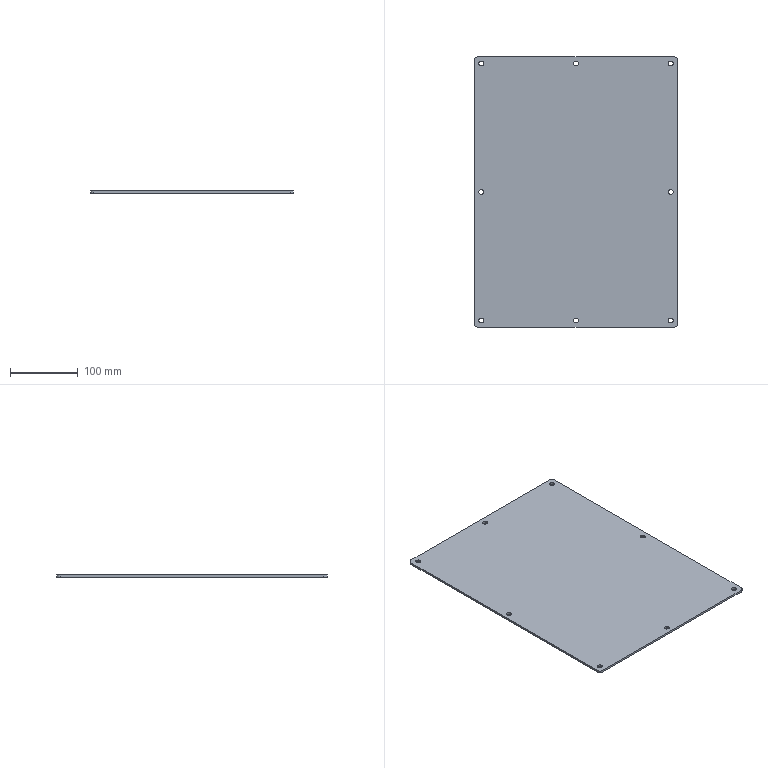Part | SolidWorks | features BaseBody 1 | 1 solid | 26 faces | box 300 x 400 x 3 mm | volume 359012 mm3 | cylinder 20 | plane 6 | commonest cylinder face diameters 7 x16 10 x4
STEP:
#1=CARTESIAN_POINT('',(136.5,-190.,0.));
#2=VERTEX_POINT('',#1);
#3=CARTESIAN_POINT('',(143.5,-190.,0.));
#4=VERTEX_POINT('',#3);
#5=CARTESIAN_POINT('',(140.,-190.,0.));
#6=DIRECTION('',(0.,0.,1.));
#7=DIRECTION('',(1.,0.,0.));
#8=AXIS2_PLACEMENT_3D('',#5,#6,#7);
#9=CIRCLE('',#8,3.5);
#10=EDGE_CURVE('',#2,#4,#9,.T.);
#11=ORIENTED_EDGE('',*,*,#10,.F.);
#12=CARTESIAN_POINT('',(136.5,-190.,3.));
#13=VERTEX_POINT('',#12);
#14=CARTESIAN_POINT('',(136.5,-190.,3.));
#15=DIRECTION('',(0.,0.,1.));
#16=VECTOR('',#15,1000.);
#17=LINE('',#14,#16);
#18=EDGE_CURVE('',#2,#13,#17,.T.);
#19=ORIENTED_EDGE('',*,*,#18,.T.);
#20=CARTESIAN_POINT('',(143.5,-190.,3.));
#21=VERTEX_POINT('',#20);
#22=CARTESIAN_POINT('',(140.,-190.,3.));
#23=DIRECTION('',(0.,0.,1.));
#24=DIRECTION('',(1.,0.,0.));
#25=AXIS2_PLACEMENT_3D('',#22,#23,#24);
#26=CIRCLE('',#25,3.5);
#27=EDGE_CURVE('',#13,#21,#26,.T.);
#28=ORIENTED_EDGE('',*,*,#27,.T.);
#29=CARTESIAN_POINT('',(143.5,-190.,3.));
#30=DIRECTION('',(0.,0.,1.));
#31=VECTOR('',#30,1000.);
#32=LINE('',#29,#31);
#33=EDGE_CURVE('',#4,#21,#32,.T.);
#34=ORIENTED_EDGE('',*,*,#33,.F.);
#35=EDGE_LOOP('',(#11,#19,#28,#34));
#36=FACE_OUTER_BOUND('',#35,.T.);
#37=CARTESIAN_POINT('',(140.,-190.,3.));
#38=DIRECTION('',(0.,0.,1.));
#39=DIRECTION('',(1.,0.,0.));
#40=AXIS2_PLACEMENT_3D('',#37,#38,#39);
#41=CYLINDRICAL_SURFACE('',#40,3.5);
#42=ADVANCED_FACE('',(#36),#41,.F.);
#43=CARTESIAN_POINT('',(-143.5,190.,0.));
#44=VERTEX_POINT('',#43);
#45=CARTESIAN_POINT('',(-136.5,190.,0.));
#46=VERTEX_POINT('',#45);
#47=CARTESIAN_POINT('',(-140.,190.,0.));
#48=DIRECTION('',(0.,0.,1.));
#49=DIRECTION('',(1.,0.,0.));
#50=AXIS2_PLACEMENT_3D('',#47,#48,#49);
#51=CIRCLE('',#50,3.5);
#52=EDGE_CURVE('',#44,#46,#51,.T.);
#53=ORIENTED_EDGE('',*,*,#52,.F.);
#54=CARTESIAN_POINT('',(-143.5,190.,3.));
#55=VERTEX_POINT('',#54);
#56=CARTESIAN_POINT('',(-143.5,190.,3.));
#57=DIRECTION('',(0.,0.,1.));
#58=VECTOR('',#57,1000.);
#59=LINE('',#56,#58);
#60=EDGE_CURVE('',#44,#55,#59,.T.);
#61=ORIENTED_EDGE('',*,*,#60,.T.);
#62=CARTESIAN_POINT('',(-136.5,190.,3.));
#63=VERTEX_POINT('',#62);
#64=CARTESIAN_POINT('',(-140.,190.,3.));
#65=DIRECTION('',(0.,0.,1.));
#66=DIRECTION('',(1.,0.,0.));
#67=AXIS2_PLACEMENT_3D('',#64,#65,#66);
#68=CIRCLE('',#67,3.5);
#69=EDGE_CURVE('',#55,#63,#68,.T.);
#70=ORIENTED_EDGE('',*,*,#69,.T.);
#71=CARTESIAN_POINT('',(-136.5,190.,3.));
#72=DIRECTION('',(0.,0.,1.));
#73=VECTOR('',#72,1000.);
#74=LINE('',#71,#73);
#75=EDGE_CURVE('',#46,#63,#74,.T.);
#76=ORIENTED_EDGE('',*,*,#75,.F.);
#77=EDGE_LOOP('',(#53,#61,#70,#76));
#78=FACE_OUTER_BOUND('',#77,.T.);
#79=CARTESIAN_POINT('',(-140.,190.,3.));
#80=DIRECTION('',(0.,0.,1.));
#81=DIRECTION('',(1.,0.,0.));
#82=AXIS2_PLACEMENT_3D('',#79,#80,#81);
#83=CYLINDRICAL_SURFACE('',#82,3.5);
#84=ADVANCED_FACE('',(#78),#83,.F.);
#85=CARTESIAN_POINT('',(-143.5,-190.,0.));
#86=VERTEX_POINT('',#85);
#87=CARTESIAN_POINT('',(-136.5,-190.,0.));
#88=VERTEX_POINT('',#87);
#89=CARTESIAN_POINT('',(-140.,-190.,0.));
#90=DIRECTION('',(0.,0.,1.));
#91=DIRECTION('',(1.,0.,0.));
#92=AXIS2_PLACEMENT_3D('',#89,#90,#91);
#93=CIRCLE('',#92,3.5);
#94=EDGE_CURVE('',#86,#88,#93,.T.);
#95=ORIENTED_EDGE('',*,*,#94,.F.);
#96=CARTESIAN_POINT('',(-143.5,-190.,3.));
#97=VERTEX_POINT('',#96);
#98=CARTESIAN_POINT('',(-143.5,-190.,3.));
#99=DIRECTION('',(0.,0.,1.));
#100=VECTOR('',#99,1000.);
#101=LINE('',#98,#100);
#102=EDGE_CURVE('',#86,#97,#101,.T.);
#103=ORIENTED_EDGE('',*,*,#102,.T.);
#104=CARTESIAN_POINT('',(-136.5,-190.,3.));
#105=VERTEX_POINT('',#104);
#106=CARTESIAN_POINT('',(-140.,-190.,3.));
#107=DIRECTION('',(0.,0.,1.));
#108=DIRECTION('',(1.,0.,0.));
#109=AXIS2_PLACEMENT_3D('',#106,#107,#108);
#110=CIRCLE('',#109,3.5);
#111=EDGE_CURVE('',#97,#105,#110,.T.);
#112=ORIENTED_EDGE('',*,*,#111,.T.);
#113=CARTESIAN_POINT('',(-136.5,-190.,3.));
#114=DIRECTION('',(0.,0.,1.));
#115=VECTOR('',#114,1000.);
#116=LINE('',#113,#115);
#117=EDGE_CURVE('',#88,#105,#116,.T.);
#118=ORIENTED_EDGE('',*,*,#117,.F.);
#119=EDGE_LOOP('',(#95,#103,#112,#118));
#120=FACE_OUTER_BOUND('',#119,.T.);
#121=CARTESIAN_POINT('',(-140.,-190.,3.));
#122=DIRECTION('',(0.,0.,1.));
#123=DIRECTION('',(1.,0.,0.));
#124=AXIS2_PLACEMENT_3D('',#121,#122,#123);
#125=CYLINDRICAL_SURFACE('',#124,3.5);
#126=ADVANCED_FACE('',(#120),#125,.F.);
#127=CARTESIAN_POINT('',(136.5,190.,0.));
#128=VERTEX_POINT('',#127);
#129=CARTESIAN_POINT('',(143.5,190.,0.));
#130=VERTEX_POINT('',#129);
#131=CARTESIAN_POINT('',(140.,190.,0.));
#132=DIRECTION('',(0.,0.,1.));
#133=DIRECTION('',(1.,0.,0.));
#134=AXIS2_PLACEMENT_3D('',#131,#132,#133);
#135=CIRCLE('',#134,3.5);
#136=EDGE_CURVE('',#128,#130,#135,.T.);
#137=ORIENTED_EDGE('',*,*,#136,.F.);
#138=CARTESIAN_POINT('',(136.5,190.,3.));
#139=VERTEX_POINT('',#138);
#140=CARTESIAN_POINT('',(136.5,190.,3.));
#141=DIRECTION('',(0.,0.,1.));
#142=VECTOR('',#141,1000.);
#143=LINE('',#140,#142);
#144=EDGE_CURVE('',#128,#139,#143,.T.);
#145=ORIENTED_EDGE('',*,*,#144,.T.);
#146=CARTESIAN_POINT('',(143.5,190.,3.));
#147=VERTEX_POINT('',#146);
#148=CARTESIAN_POINT('',(140.,190.,3.));
#149=DIRECTION('',(0.,0.,1.));
#150=DIRECTION('',(1.,0.,0.));
#151=AXIS2_PLACEMENT_3D('',#148,#149,#150);
#152=CIRCLE('',#151,3.5);
#153=EDGE_CURVE('',#139,#147,#152,.T.);
#154=ORIENTED_EDGE('',*,*,#153,.T.);
#155=CARTESIAN_POINT('',(143.5,190.,3.));
#156=DIRECTION('',(0.,0.,1.));
#157=VECTOR('',#156,1000.);
#158=LINE('',#155,#157);
#159=EDGE_CURVE('',#130,#147,#158,.T.);
#160=ORIENTED_EDGE('',*,*,#159,.F.);
#161=EDGE_LOOP('',(#137,#145,#154,#160));
#162=FACE_OUTER_BOUND('',#161,.T.);
#163=CARTESIAN_POINT('',(140.,190.,3.));
#164=DIRECTION('',(0.,0.,1.));
#165=DIRECTION('',(1.,0.,0.));
#166=AXIS2_PLACEMENT_3D('',#163,#164,#165);
#167=CYLINDRICAL_SURFACE('',#166,3.5);
#168=ADVANCED_FACE('',(#162),#167,.F.);
#169=CARTESIAN_POINT('',(-3.5,190.,0.));
#170=VERTEX_POINT('',#169);
#171=CARTESIAN_POINT('',(3.5,190.,0.));
#172=VERTEX_POINT('',#171);
#173=CARTESIAN_POINT('',(0.,190.,0.));
#174=DIRECTION('',(0.,0.,1.));
#175=DIRECTION('',(1.,0.,0.));
#176=AXIS2_PLACEMENT_3D('',#173,#174,#175);
#177=CIRCLE('',#176,3.5);
#178=EDGE_CURVE('',#170,#172,#177,.T.);
#179=ORIENTED_EDGE('',*,*,#178,.F.);
#180=CARTESIAN_POINT('',(-3.5,190.,3.));
#181=VERTEX_POINT('',#180);
#182=CARTESIAN_POINT('',(-3.5,190.,3.));
#183=DIRECTION('',(0.,0.,1.));
#184=VECTOR('',#183,1000.);
#185=LINE('',#182,#184);
#186=EDGE_CURVE('',#170,#181,#185,.T.);
#187=ORIENTED_EDGE('',*,*,#186,.T.);
#188=CARTESIAN_POINT('',(3.5,190.,3.));
#189=VERTEX_POINT('',#188);
#190=CARTESIAN_POINT('',(0.,190.,3.));
#191=DIRECTION('',(0.,0.,1.));
#192=DIRECTION('',(1.,0.,0.));
#193=AXIS2_PLACEMENT_3D('',#190,#191,#192);
#194=CIRCLE('',#193,3.5);
#195=EDGE_CURVE('',#181,#189,#194,.T.);
#196=ORIENTED_EDGE('',*,*,#195,.T.);
#197=CARTESIAN_POINT('',(3.5,190.,3.));
#198=DIRECTION('',(0.,0.,1.));
#199=VECTOR('',#198,1000.);
#200=LINE('',#197,#199);
#201=EDGE_CURVE('',#172,#189,#200,.T.);
#202=ORIENTED_EDGE('',*,*,#201,.F.);
#203=EDGE_LOOP('',(#179,#187,#196,#202));
#204=FACE_OUTER_BOUND('',#203,.T.);
#205=CARTESIAN_POINT('',(0.,190.,3.));
#206=DIRECTION('',(0.,0.,1.));
#207=DIRECTION('',(1.,0.,0.));
#208=AXIS2_PLACEMENT_3D('',#205,#206,#207);
#209=CYLINDRICAL_SURFACE('',#208,3.5);
#210=ADVANCED_FACE('',(#204),#209,.F.);
#211=CARTESIAN_POINT('',(-3.5,-190.,0.));
#212=VERTEX_POINT('',#211);
#213=CARTESIAN_POINT('',(3.5,-190.,0.));
#214=VERTEX_POINT('',#213);
#215=CARTESIAN_POINT('',(0.,-190.,0.));
#216=DIRECTION('',(0.,0.,1.));
#217=DIRECTION('',(1.,0.,0.));
#218=AXIS2_PLACEMENT_3D('',#215,#216,#217);
#219=CIRCLE('',#218,3.5);
#220=EDGE_CURVE('',#212,#214,#219,.T.);
#221=ORIENTED_EDGE('',*,*,#220,.F.);
#222=CARTESIAN_POINT('',(-3.5,-190.,3.));
#223=VERTEX_POINT('',#222);
#224=CARTESIAN_POINT('',(-3.5,-190.,3.));
#225=DIRECTION('',(0.,0.,1.));
#226=VECTOR('',#225,1000.);
#227=LINE('',#224,#226);
#228=EDGE_CURVE('',#212,#223,#227,.T.);
#229=ORIENTED_EDGE('',*,*,#228,.T.);
#230=CARTESIAN_POINT('',(3.5,-190.,3.));
#231=VERTEX_POINT('',#230);
#232=CARTESIAN_POINT('',(0.,-190.,3.));
#233=DIRECTION('',(0.,0.,1.));
#234=DIRECTION('',(1.,0.,0.));
#235=AXIS2_PLACEMENT_3D('',#232,#233,#234);
#236=CIRCLE('',#235,3.5);
#237=EDGE_CURVE('',#223,#231,#236,.T.);
#238=ORIENTED_EDGE('',*,*,#237,.T.);
#239=CARTESIAN_POINT('',(3.5,-190.,3.));
#240=DIRECTION('',(0.,0.,1.));
#241=VECTOR('',#240,1000.);
#242=LINE('',#239,#241);
#243=EDGE_CURVE('',#214,#231,#242,.T.);
#244=ORIENTED_EDGE('',*,*,#243,.F.);
#245=EDGE_LOOP('',(#221,#229,#238,#244));
#246=FACE_OUTER_BOUND('',#245,.T.);
#247=CARTESIAN_POINT('',(0.,-190.,3.));
#248=DIRECTION('',(0.,0.,1.));
#249=DIRECTION('',(1.,0.,0.));
#250=AXIS2_PLACEMENT_3D('',#247,#248,#249);
#251=CYLINDRICAL_SURFACE('',#250,3.5);
#252=ADVANCED_FACE('',(#246),#251,.F.);
#253=CARTESIAN_POINT('',(-143.5,0.,0.));
#254=VERTEX_POINT('',#253);
#255=CARTESIAN_POINT('',(-136.5,0.,0.));
#256=VERTEX_POINT('',#255);
#257=CARTESIAN_POINT('',(-140.,0.,0.));
#258=DIRECTION('',(0.,0.,1.));
#259=DIRECTION('',(1.,0.,0.));
#260=AXIS2_PLACEMENT_3D('',#257,#258,#259);
#261=CIRCLE('',#260,3.5);
#262=EDGE_CURVE('',#254,#256,#261,.T.);
#263=ORIENTED_EDGE('',*,*,#262,.F.);
#264=CARTESIAN_POINT('',(-143.5,0.,3.));
#265=VERTEX_POINT('',#264);
#266=CARTESIAN_POINT('',(-143.5,0.,3.));
#267=DIRECTION('',(0.,0.,1.));
#268=VECTOR('',#267,1000.);
#269=LINE('',#266,#268);
#270=EDGE_CURVE('',#254,#265,#269,.T.);
#271=ORIENTED_EDGE('',*,*,#270,.T.);
#272=CARTESIAN_POINT('',(-136.5,0.,3.));
#273=VERTEX_POINT('',#272);
#274=CARTESIAN_POINT('',(-140.,0.,3.));
#275=DIRECTION('',(0.,0.,1.));
#276=DIRECTION('',(1.,0.,0.));
#277=AXIS2_PLACEMENT_3D('',#274,#275,#276);
#278=CIRCLE('',#277,3.5);
#279=EDGE_CURVE('',#265,#273,#278,.T.);
#280=ORIENTED_EDGE('',*,*,#279,.T.);
#281=CARTESIAN_POINT('',(-136.5,0.,3.));
#282=DIRECTION('',(0.,0.,1.));
#283=VECTOR('',#282,1000.);
#284=LINE('',#281,#283);
#285=EDGE_CURVE('',#256,#273,#284,.T.);
#286=ORIENTED_EDGE('',*,*,#285,.F.);
#287=EDGE_LOOP('',(#263,#271,#280,#286));
#288=FACE_OUTER_BOUND('',#287,.T.);
#289=CARTESIAN_POINT('',(-140.,0.,3.));
#290=DIRECTION('',(0.,0.,1.));
#291=DIRECTION('',(1.,0.,0.));
#292=AXIS2_PLACEMENT_3D('',#289,#290,#291);
#293=CYLINDRICAL_SURFACE('',#292,3.5);
#294=ADVANCED_FACE('',(#288),#293,.F.);
#295=CARTESIAN_POINT('',(136.5,0.,0.));
#296=VERTEX_POINT('',#295);
#297=CARTESIAN_POINT('',(143.5,0.,0.));
#298=VERTEX_POINT('',#297);
#299=CARTESIAN_POINT('',(140.,0.,0.));
#300=DIRECTION('',(0.,0.,1.));
#301=DIRECTION('',(1.,0.,0.));
#302=AXIS2_PLACEMENT_3D('',#299,#300,#301);
#303=CIRCLE('',#302,3.5);
#304=EDGE_CURVE('',#296,#298,#303,.T.);
#305=ORIENTED_EDGE('',*,*,#304,.F.);
#306=CARTESIAN_POINT('',(136.5,0.,3.));
#307=VERTEX_POINT('',#306);
#308=CARTESIAN_POINT('',(136.5,0.,3.));
#309=DIRECTION('',(0.,0.,1.));
#310=VECTOR('',#309,1000.);
#311=LINE('',#308,#310);
#312=EDGE_CURVE('',#296,#307,#311,.T.);
#313=ORIENTED_EDGE('',*,*,#312,.T.);
#314=CARTESIAN_POINT('',(143.5,0.,3.));
#315=VERTEX_POINT('',#314);
#316=CARTESIAN_POINT('',(140.,0.,3.));
#317=DIRECTION('',(0.,0.,1.));
#318=DIRECTION('',(1.,0.,0.));
#319=AXIS2_PLACEMENT_3D('',#316,#317,#318);
#320=CIRCLE('',#319,3.5);
#321=EDGE_CURVE('',#307,#315,#320,.T.);
#322=ORIENTED_EDGE('',*,*,#321,.T.);
#323=CARTESIAN_POINT('',(143.5,0.,3.));
#324=DIRECTION('',(0.,0.,1.));
#325=VECTOR('',#324,1000.);
#326=LINE('',#323,#325);
#327=EDGE_CURVE('',#298,#315,#326,.T.);
#328=ORIENTED_EDGE('',*,*,#327,.F.);
#329=EDGE_LOOP('',(#305,#313,#322,#328));
#330=FACE_OUTER_BOUND('',#329,.T.);
#331=CARTESIAN_POINT('',(140.,0.,3.));
#332=DIRECTION('',(0.,0.,1.));
#333=DIRECTION('',(1.,0.,0.));
#334=AXIS2_PLACEMENT_3D('',#331,#332,#333);
#335=CYLINDRICAL_SURFACE('',#334,3.5);
#336=ADVANCED_FACE('',(#330),#335,.F.);
#337=CARTESIAN_POINT('',(-150.,-195.,0.));
#338=VERTEX_POINT('',#337);
#339=CARTESIAN_POINT('',(-145.,-200.,0.));
#340=VERTEX_POINT('',#339);
#341=CARTESIAN_POINT('',(-145.,-195.,0.));
#342=DIRECTION('',(0.,0.,1.));
#343=DIRECTION('',(1.,0.,0.));
#344=AXIS2_PLACEMENT_3D('',#341,#342,#343);
#345=CIRCLE('',#344,5.);
#346=EDGE_CURVE('',#338,#340,#345,.T.);
#347=ORIENTED_EDGE('',*,*,#346,.T.);
#348=CARTESIAN_POINT('',(-145.,-200.,3.));
#349=VERTEX_POINT('',#348);
#350=CARTESIAN_POINT('',(-145.,-200.,3.));
#351=DIRECTION('',(0.,0.,-1.));
#352=VECTOR('',#351,1000.);
#353=LINE('',#350,#352);
#354=EDGE_CURVE('',#349,#340,#353,.T.);
#355=ORIENTED_EDGE('',*,*,#354,.F.);
#356=CARTESIAN_POINT('',(-150.,-195.,3.));
#357=VERTEX_POINT('',#356);
#358=CARTESIAN_POINT('',(-145.,-195.,3.));
#359=DIRECTION('',(0.,0.,1.));
#360=DIRECTION('',(1.,0.,0.));
#361=AXIS2_PLACEMENT_3D('',#358,#359,#360);
#362=CIRCLE('',#361,5.);
#363=EDGE_CURVE('',#357,#349,#362,.T.);
#364=ORIENTED_EDGE('',*,*,#363,.F.);
#365=CARTESIAN_POINT('',(-150.,-195.,3.));
#366=DIRECTION('',(0.,0.,-1.));
#367=VECTOR('',#366,1000.);
#368=LINE('',#365,#367);
#369=EDGE_CURVE('',#357,#338,#368,.T.);
#370=ORIENTED_EDGE('',*,*,#369,.T.);
#371=EDGE_LOOP('',(#347,#355,#364,#370));
#372=FACE_OUTER_BOUND('',#371,.T.);
#373=CARTESIAN_POINT('',(-145.,-195.,3.));
#374=DIRECTION('',(0.,0.,-1.));
#375=DIRECTION('',(-1.,0.,0.));
#376=AXIS2_PLACEMENT_3D('',#373,#374,#375);
#377=CYLINDRICAL_SURFACE('',#376,5.);
#378=ADVANCED_FACE('',(#372),#377,.T.);
#379=CARTESIAN_POINT('',(145.,-200.,0.));
#380=VERTEX_POINT('',#379);
#381=CARTESIAN_POINT('',(-145.,-200.,0.));
#382=DIRECTION('',(1.,0.,0.));
#383=VECTOR('',#382,1000.);
#384=LINE('',#381,#383);
#385=EDGE_CURVE('',#340,#380,#384,.T.);
#386=ORIENTED_EDGE('',*,*,#385,.T.);
#387=CARTESIAN_POINT('',(145.,-200.,3.));
#388=VERTEX_POINT('',#387);
#389=CARTESIAN_POINT('',(145.,-200.,3.));
#390=DIRECTION('',(0.,0.,-1.));
#391=VECTOR('',#390,1000.);
#392=LINE('',#389,#391);
#393=EDGE_CURVE('',#388,#380,#392,.T.);
#394=ORIENTED_EDGE('',*,*,#393,.F.);
#395=CARTESIAN_POINT('',(-145.,-200.,3.));
#396=DIRECTION('',(1.,0.,0.));
#397=VECTOR('',#396,1000.);
#398=LINE('',#395,#397);
#399=EDGE_CURVE('',#349,#388,#398,.T.);
#400=ORIENTED_EDGE('',*,*,#399,.F.);
#401=ORIENTED_EDGE('',*,*,#354,.T.);
#402=EDGE_LOOP('',(#386,#394,#400,#401));
#403=FACE_OUTER_BOUND('',#402,.T.);
#404=CARTESIAN_POINT('',(-145.,-200.,3.));
#405=DIRECTION('',(0.,1.,0.));
#406=DIRECTION('',(0.,0.,1.));
#407=AXIS2_PLACEMENT_3D('',#404,#405,#406);
#408=PLANE('',#407);
#409=ADVANCED_FACE('',(#403),#408,.F.);
#410=CARTESIAN_POINT('',(150.,-195.,0.));
#411=VERTEX_POINT('',#410);
#412=CARTESIAN_POINT('',(145.,-195.,0.));
#413=DIRECTION('',(0.,0.,1.));
#414=DIRECTION('',(1.,0.,0.));
#415=AXIS2_PLACEMENT_3D('',#412,#413,#414);
#416=CIRCLE('',#415,5.);
#417=EDGE_CURVE('',#380,#411,#416,.T.);
#418=ORIENTED_EDGE('',*,*,#417,.T.);
#419=CARTESIAN_POINT('',(150.,-195.,3.));
#420=VERTEX_POINT('',#419);
#421=CARTESIAN_POINT('',(150.,-195.,3.));
#422=DIRECTION('',(0.,0.,-1.));
#423=VECTOR('',#422,1000.);
#424=LINE('',#421,#423);
#425=EDGE_CURVE('',#420,#411,#424,.T.);
#426=ORIENTED_EDGE('',*,*,#425,.F.);
#427=CARTESIAN_POINT('',(145.,-195.,3.));
#428=DIRECTION('',(0.,0.,1.));
#429=DIRECTION('',(1.,0.,0.));
#430=AXIS2_PLACEMENT_3D('',#427,#428,#429);
#431=CIRCLE('',#430,5.);
#432=EDGE_CURVE('',#388,#420,#431,.T.);
#433=ORIENTED_EDGE('',*,*,#432,.F.);
#434=ORIENTED_EDGE('',*,*,#393,.T.);
#435=EDGE_LOOP('',(#418,#426,#433,#434));
#436=FACE_OUTER_BOUND('',#435,.T.);
#437=CARTESIAN_POINT('',(145.,-195.,3.));
#438=DIRECTION('',(0.,0.,-1.));
#439=DIRECTION('',(-1.,0.,0.));
#440=AXIS2_PLACEMENT_3D('',#437,#438,#439);
#441=CYLINDRICAL_SURFACE('',#440,5.);
#442=ADVANCED_FACE('',(#436),#441,.T.);
#443=CARTESIAN_POINT('',(150.,195.,0.));
#444=VERTEX_POINT('',#443);
#445=CARTESIAN_POINT('',(150.,195.,0.));
#446=DIRECTION('',(0.,1.,0.));
#447=VECTOR('',#446,1000.);
#448=LINE('',#445,#447);
#449=EDGE_CURVE('',#411,#444,#448,.T.);
#450=ORIENTED_EDGE('',*,*,#449,.T.);
#451=CARTESIAN_POINT('',(150.,195.,3.));
#452=VERTEX_POINT('',#451);
#453=CARTESIAN_POINT('',(150.,195.,3.));
#454=DIRECTION('',(0.,0.,-1.));
#455=VECTOR('',#454,1000.);
#456=LINE('',#453,#455);
#457=EDGE_CURVE('',#452,#444,#456,.T.);
#458=ORIENTED_EDGE('',*,*,#457,.F.);
#459=CARTESIAN_POINT('',(150.,195.,3.));
#460=DIRECTION('',(0.,1.,0.));
#461=VECTOR('',#460,1000.);
#462=LINE('',#459,#461);
#463=EDGE_CURVE('',#420,#452,#462,.T.);
#464=ORIENTED_EDGE('',*,*,#463,.F.);
#465=ORIENTED_EDGE('',*,*,#425,.T.);
#466=EDGE_LOOP('',(#450,#458,#464,#465));
#467=FACE_OUTER_BOUND('',#466,.T.);
#468=CARTESIAN_POINT('',(150.,195.,3.));
#469=DIRECTION('',(-1.,0.,0.));
#470=DIRECTION('',(0.,-1.,0.));
#471=AXIS2_PLACEMENT_3D('',#468,#469,#470);
#472=PLANE('',#471);
#473=ADVANCED_FACE('',(#467),#472,.F.);
#474=CARTESIAN_POINT('',(145.,200.,0.));
#475=VERTEX_POINT('',#474);
#476=CARTESIAN_POINT('',(145.,195.,0.));
#477=DIRECTION('',(0.,0.,1.));
#478=DIRECTION('',(-1.,0.,0.));
#479=AXIS2_PLACEMENT_3D('',#476,#477,#478);
#480=CIRCLE('',#479,5.);
#481=EDGE_CURVE('',#444,#475,#480,.T.);
#482=ORIENTED_EDGE('',*,*,#481,.T.);
#483=CARTESIAN_POINT('',(145.,200.,3.));
#484=VERTEX_POINT('',#483);
#485=CARTESIAN_POINT('',(145.,200.,3.));
#486=DIRECTION('',(0.,0.,-1.));
#487=VECTOR('',#486,1000.);
#488=LINE('',#485,#487);
#489=EDGE_CURVE('',#484,#475,#488,.T.);
#490=ORIENTED_EDGE('',*,*,#489,.F.);
#491=CARTESIAN_POINT('',(145.,195.,3.));
#492=DIRECTION('',(0.,0.,1.));
#493=DIRECTION('',(-1.,0.,0.));
#494=AXIS2_PLACEMENT_3D('',#491,#492,#493);
#495=CIRCLE('',#494,5.);
#496=EDGE_CURVE('',#452,#484,#495,.T.);
#497=ORIENTED_EDGE('',*,*,#496,.F.);
#498=ORIENTED_EDGE('',*,*,#457,.T.);
#499=EDGE_LOOP('',(#482,#490,#497,#498));
#500=FACE_OUTER_BOUND('',#499,.T.);
#501=CARTESIAN_POINT('',(145.,195.,3.));
#502=DIRECTION('',(0.,0.,-1.));
#503=DIRECTION('',(-1.,0.,0.));
#504=AXIS2_PLACEMENT_3D('',#501,#502,#503);
#505=CYLINDRICAL_SURFACE('',#504,5.);
#506=ADVANCED_FACE('',(#500),#505,.T.);
#507=CARTESIAN_POINT('',(-145.,200.,0.));
#508=VERTEX_POINT('',#507);
#509=CARTESIAN_POINT('',(-145.,200.,0.));
#510=DIRECTION('',(-1.,0.,0.));
#511=VECTOR('',#510,1000.);
#512=LINE('',#509,#511);
#513=EDGE_CURVE('',#475,#508,#512,.T.);
#514=ORIENTED_EDGE('',*,*,#513,.T.);
#515=CARTESIAN_POINT('',(-145.,200.,3.));
#516=VERTEX_POINT('',#515);
#517=CARTESIAN_POINT('',(-145.,200.,3.));
#518=DIRECTION('',(0.,0.,-1.));
#519=VECTOR('',#518,1000.);
#520=LINE('',#517,#519);
#521=EDGE_CURVE('',#516,#508,#520,.T.);
#522=ORIENTED_EDGE('',*,*,#521,.F.);
#523=CARTESIAN_POINT('',(-145.,200.,3.));
#524=DIRECTION('',(-1.,0.,0.));
#525=VECTOR('',#524,1000.);
#526=LINE('',#523,#525);
#527=EDGE_CURVE('',#484,#516,#526,.T.);
#528=ORIENTED_EDGE('',*,*,#527,.F.);
#529=ORIENTED_EDGE('',*,*,#489,.T.);
#530=EDGE_LOOP('',(#514,#522,#528,#529));
#531=FACE_OUTER_BOUND('',#530,.T.);
#532=CARTESIAN_POINT('',(-145.,200.,3.));
#533=DIRECTION('',(0.,-1.,0.));
#534=DIRECTION('',(0.,0.,-1.));
#535=AXIS2_PLACEMENT_3D('',#532,#533,#534);
#536=PLANE('',#535);
#537=ADVANCED_FACE('',(#531),#536,.F.);
#538=CARTESIAN_POINT('',(-150.,195.,0.));
#539=VERTEX_POINT('',#538);
#540=CARTESIAN_POINT('',(-145.,195.,0.));
#541=DIRECTION('',(0.,0.,1.));
#542=DIRECTION('',(1.,0.,0.));
#543=AXIS2_PLACEMENT_3D('',#540,#541,#542);
#544=CIRCLE('',#543,5.);
#545=EDGE_CURVE('',#508,#539,#544,.T.);
#546=ORIENTED_EDGE('',*,*,#545,.T.);
#547=CARTESIAN_POINT('',(-150.,195.,3.));
#548=VERTEX_POINT('',#547);
#549=CARTESIAN_POINT('',(-150.,195.,3.));
#550=DIRECTION('',(0.,0.,-1.));
#551=VECTOR('',#550,1000.);
#552=LINE('',#549,#551);
#553=EDGE_CURVE('',#548,#539,#552,.T.);
#554=ORIENTED_EDGE('',*,*,#553,.F.);
#555=CARTESIAN_POINT('',(-145.,195.,3.));
#556=DIRECTION('',(0.,0.,1.));
#557=DIRECTION('',(1.,0.,0.));
#558=AXIS2_PLACEMENT_3D('',#555,#556,#557);
#559=CIRCLE('',#558,5.);
#560=EDGE_CURVE('',#516,#548,#559,.T.);
#561=ORIENTED_EDGE('',*,*,#560,.F.);
#562=ORIENTED_EDGE('',*,*,#521,.T.);
#563=EDGE_LOOP('',(#546,#554,#561,#562));
#564=FACE_OUTER_BOUND('',#563,.T.);
#565=CARTESIAN_POINT('',(-145.,195.,3.));
#566=DIRECTION('',(0.,0.,-1.));
#567=DIRECTION('',(-1.,0.,0.));
#568=AXIS2_PLACEMENT_3D('',#565,#566,#567);
#569=CYLINDRICAL_SURFACE('',#568,5.);
#570=ADVANCED_FACE('',(#564),#569,.T.);
#571=CARTESIAN_POINT('',(-150.,195.,0.));
#572=DIRECTION('',(0.,-1.,0.));
#573=VECTOR('',#572,1000.);
#574=LINE('',#571,#573);
#575=EDGE_CURVE('',#539,#338,#574,.T.);
#576=ORIENTED_EDGE('',*,*,#575,.T.);
#577=ORIENTED_EDGE('',*,*,#369,.F.);
#578=CARTESIAN_POINT('',(-150.,195.,3.));
#579=DIRECTION('',(0.,-1.,0.));
#580=VECTOR('',#579,1000.);
#581=LINE('',#578,#580);
#582=EDGE_CURVE('',#548,#357,#581,.T.);
#583=ORIENTED_EDGE('',*,*,#582,.F.);
#584=ORIENTED_EDGE('',*,*,#553,.T.);
#585=EDGE_LOOP('',(#576,#577,#583,#584));
#586=FACE_OUTER_BOUND('',#585,.T.);
#587=CARTESIAN_POINT('',(-150.,195.,3.));
#588=DIRECTION('',(1.,0.,0.));
#589=DIRECTION('',(0.,1.,0.));
#590=AXIS2_PLACEMENT_3D('',#587,#588,#589);
#591=PLANE('',#590);
#592=ADVANCED_FACE('',(#586),#591,.F.);
#593=CARTESIAN_POINT('',(140.,-190.,3.));
#594=DIRECTION('',(0.,0.,1.));
#595=DIRECTION('',(1.,0.,0.));
#596=AXIS2_PLACEMENT_3D('',#593,#594,#595);
#597=CIRCLE('',#596,3.5);
#598=EDGE_CURVE('',#21,#13,#597,.T.);
#599=ORIENTED_EDGE('',*,*,#598,.F.);
#600=ORIENTED_EDGE('',*,*,#27,.F.);
#601=EDGE_LOOP('',(#599,#600));
#602=FACE_BOUND('',#601,.T.);
#603=CARTESIAN_POINT('',(-140.,190.,3.));
#604=DIRECTION('',(0.,0.,1.));
#605=DIRECTION('',(1.,0.,0.));
#606=AXIS2_PLACEMENT_3D('',#603,#604,#605);
#607=CIRCLE('',#606,3.5);
#608=EDGE_CURVE('',#63,#55,#607,.T.);
#609=ORIENTED_EDGE('',*,*,#608,.F.);
#610=ORIENTED_EDGE('',*,*,#69,.F.);
#611=EDGE_LOOP('',(#609,#610));
#612=FACE_BOUND('',#611,.T.);
#613=CARTESIAN_POINT('',(-140.,-190.,3.));
#614=DIRECTION('',(0.,0.,1.));
#615=DIRECTION('',(1.,0.,0.));
#616=AXIS2_PLACEMENT_3D('',#613,#614,#615);
#617=CIRCLE('',#616,3.5);
#618=EDGE_CURVE('',#105,#97,#617,.T.);
#619=ORIENTED_EDGE('',*,*,#618,.F.);
#620=ORIENTED_EDGE('',*,*,#111,.F.);
#621=EDGE_LOOP('',(#619,#620));
#622=FACE_BOUND('',#621,.T.);
#623=CARTESIAN_POINT('',(140.,190.,3.));
#624=DIRECTION('',(0.,0.,1.));
#625=DIRECTION('',(1.,0.,0.));
#626=AXIS2_PLACEMENT_3D('',#623,#624,#625);
#627=CIRCLE('',#626,3.5);
#628=EDGE_CURVE('',#147,#139,#627,.T.);
#629=ORIENTED_EDGE('',*,*,#628,.F.);
#630=ORIENTED_EDGE('',*,*,#153,.F.);
#631=EDGE_LOOP('',(#629,#630));
#632=FACE_BOUND('',#631,.T.);
#633=CARTESIAN_POINT('',(0.,190.,3.));
#634=DIRECTION('',(0.,0.,1.));
#635=DIRECTION('',(1.,0.,0.));
#636=AXIS2_PLACEMENT_3D('',#633,#634,#635);
#637=CIRCLE('',#636,3.5);
#638=EDGE_CURVE('',#189,#181,#637,.T.);
#639=ORIENTED_EDGE('',*,*,#638,.F.);
#640=ORIENTED_EDGE('',*,*,#195,.F.);
#641=EDGE_LOOP('',(#639,#640));
#642=FACE_BOUND('',#641,.T.);
#643=CARTESIAN_POINT('',(0.,-190.,3.));
#644=DIRECTION('',(0.,0.,1.));
#645=DIRECTION('',(1.,0.,0.));
#646=AXIS2_PLACEMENT_3D('',#643,#644,#645);
#647=CIRCLE('',#646,3.5);
#648=EDGE_CURVE('',#231,#223,#647,.T.);
#649=ORIENTED_EDGE('',*,*,#648,.F.);
#650=ORIENTED_EDGE('',*,*,#237,.F.);
#651=EDGE_LOOP('',(#649,#650));
#652=FACE_BOUND('',#651,.T.);
#653=CARTESIAN_POINT('',(-140.,0.,3.));
#654=DIRECTION('',(0.,0.,1.));
#655=DIRECTION('',(1.,0.,0.));
#656=AXIS2_PLACEMENT_3D('',#653,#654,#655);
#657=CIRCLE('',#656,3.5);
#658=EDGE_CURVE('',#273,#265,#657,.T.);
#659=ORIENTED_EDGE('',*,*,#658,.F.);
#660=ORIENTED_EDGE('',*,*,#279,.F.);
#661=EDGE_LOOP('',(#659,#660));
#662=FACE_BOUND('',#661,.T.);
#663=CARTESIAN_POINT('',(140.,0.,3.));
#664=DIRECTION('',(0.,0.,1.));
#665=DIRECTION('',(1.,0.,0.));
#666=AXIS2_PLACEMENT_3D('',#663,#664,#665);
#667=CIRCLE('',#666,3.5);
#668=EDGE_CURVE('',#315,#307,#667,.T.);
#669=ORIENTED_EDGE('',*,*,#668,.F.);
#670=ORIENTED_EDGE('',*,*,#321,.F.);
#671=EDGE_LOOP('',(#669,#670));
#672=FACE_BOUND('',#671,.T.);
#673=ORIENTED_EDGE('',*,*,#363,.T.);
#674=ORIENTED_EDGE('',*,*,#399,.T.);
#675=ORIENTED_EDGE('',*,*,#432,.T.);
#676=ORIENTED_EDGE('',*,*,#463,.T.);
#677=ORIENTED_EDGE('',*,*,#496,.T.);
#678=ORIENTED_EDGE('',*,*,#527,.T.);
#679=ORIENTED_EDGE('',*,*,#560,.T.);
#680=ORIENTED_EDGE('',*,*,#582,.T.);
#681=EDGE_LOOP('',(#673,#674,#675,#676,#677,#678,#679,#680));
#682=FACE_OUTER_BOUND('',#681,.T.);
#683=CARTESIAN_POINT('',(-145.,-195.,3.));
#684=DIRECTION('',(0.,0.,1.));
#685=DIRECTION('',(1.,0.,0.));
#686=AXIS2_PLACEMENT_3D('',#683,#684,#685);
#687=PLANE('',#686);
#688=ADVANCED_FACE('',(#602,#612,#622,#632,#642,#652,#662,#672,#682),#687,.T.);
#689=CARTESIAN_POINT('',(140.,-190.,0.));
#690=DIRECTION('',(0.,0.,1.));
#691=DIRECTION('',(1.,0.,0.));
#692=AXIS2_PLACEMENT_3D('',#689,#690,#691);
#693=CIRCLE('',#692,3.5);
#694=EDGE_CURVE('',#4,#2,#693,.T.);
#695=ORIENTED_EDGE('',*,*,#694,.T.);
#696=ORIENTED_EDGE('',*,*,#10,.T.);
#697=EDGE_LOOP('',(#695,#696));
#698=FACE_BOUND('',#697,.T.);
#699=CARTESIAN_POINT('',(-140.,190.,0.));
#700=DIRECTION('',(0.,0.,1.));
#701=DIRECTION('',(1.,0.,0.));
#702=AXIS2_PLACEMENT_3D('',#699,#700,#701);
#703=CIRCLE('',#702,3.5);
#704=EDGE_CURVE('',#46,#44,#703,.T.);
#705=ORIENTED_EDGE('',*,*,#704,.T.);
#706=ORIENTED_EDGE('',*,*,#52,.T.);
#707=EDGE_LOOP('',(#705,#706));
#708=FACE_BOUND('',#707,.T.);
#709=CARTESIAN_POINT('',(-140.,-190.,0.));
#710=DIRECTION('',(0.,0.,1.));
#711=DIRECTION('',(1.,0.,0.));
#712=AXIS2_PLACEMENT_3D('',#709,#710,#711);
#713=CIRCLE('',#712,3.5);
#714=EDGE_CURVE('',#88,#86,#713,.T.);
#715=ORIENTED_EDGE('',*,*,#714,.T.);
#716=ORIENTED_EDGE('',*,*,#94,.T.);
#717=EDGE_LOOP('',(#715,#716));
#718=FACE_BOUND('',#717,.T.);
#719=CARTESIAN_POINT('',(140.,190.,0.));
#720=DIRECTION('',(0.,0.,1.));
#721=DIRECTION('',(1.,0.,0.));
#722=AXIS2_PLACEMENT_3D('',#719,#720,#721);
#723=CIRCLE('',#722,3.5);
#724=EDGE_CURVE('',#130,#128,#723,.T.);
#725=ORIENTED_EDGE('',*,*,#724,.T.);
#726=ORIENTED_EDGE('',*,*,#136,.T.);
#727=EDGE_LOOP('',(#725,#726));
#728=FACE_BOUND('',#727,.T.);
#729=CARTESIAN_POINT('',(0.,190.,0.));
#730=DIRECTION('',(0.,0.,1.));
#731=DIRECTION('',(1.,0.,0.));
#732=AXIS2_PLACEMENT_3D('',#729,#730,#731);
#733=CIRCLE('',#732,3.5);
#734=EDGE_CURVE('',#172,#170,#733,.T.);
#735=ORIENTED_EDGE('',*,*,#734,.T.);
#736=ORIENTED_EDGE('',*,*,#178,.T.);
#737=EDGE_LOOP('',(#735,#736));
#738=FACE_BOUND('',#737,.T.);
#739=CARTESIAN_POINT('',(0.,-190.,0.));
#740=DIRECTION('',(0.,0.,1.));
#741=DIRECTION('',(1.,0.,0.));
#742=AXIS2_PLACEMENT_3D('',#739,#740,#741);
#743=CIRCLE('',#742,3.5);
#744=EDGE_CURVE('',#214,#212,#743,.T.);
#745=ORIENTED_EDGE('',*,*,#744,.T.);
#746=ORIENTED_EDGE('',*,*,#220,.T.);
#747=EDGE_LOOP('',(#745,#746));
#748=FACE_BOUND('',#747,.T.);
#749=CARTESIAN_POINT('',(-140.,0.,0.));
#750=DIRECTION('',(0.,0.,1.));
#751=DIRECTION('',(1.,0.,0.));
#752=AXIS2_PLACEMENT_3D('',#749,#750,#751);
#753=CIRCLE('',#752,3.5);
#754=EDGE_CURVE('',#256,#254,#753,.T.);
#755=ORIENTED_EDGE('',*,*,#754,.T.);
#756=ORIENTED_EDGE('',*,*,#262,.T.);
#757=EDGE_LOOP('',(#755,#756));
#758=FACE_BOUND('',#757,.T.);
#759=CARTESIAN_POINT('',(140.,0.,0.));
#760=DIRECTION('',(0.,0.,1.));
#761=DIRECTION('',(1.,0.,0.));
#762=AXIS2_PLACEMENT_3D('',#759,#760,#761);
#763=CIRCLE('',#762,3.5);
#764=EDGE_CURVE('',#298,#296,#763,.T.);
#765=ORIENTED_EDGE('',*,*,#764,.T.);
#766=ORIENTED_EDGE('',*,*,#304,.T.);
#767=EDGE_LOOP('',(#765,#766));
#768=FACE_BOUND('',#767,.T.);
#769=ORIENTED_EDGE('',*,*,#346,.F.);
#770=ORIENTED_EDGE('',*,*,#575,.F.);
#771=ORIENTED_EDGE('',*,*,#545,.F.);
#772=ORIENTED_EDGE('',*,*,#513,.F.);
#773=ORIENTED_EDGE('',*,*,#481,.F.);
#774=ORIENTED_EDGE('',*,*,#449,.F.);
#775=ORIENTED_EDGE('',*,*,#417,.F.);
#776=ORIENTED_EDGE('',*,*,#385,.F.);
#777=EDGE_LOOP('',(#769,#770,#771,#772,#773,#774,#775,#776));
#778=FACE_OUTER_BOUND('',#777,.T.);
#779=CARTESIAN_POINT('',(-145.,-195.,0.));
#780=DIRECTION('',(0.,0.,1.));
#781=DIRECTION('',(1.,0.,0.));
#782=AXIS2_PLACEMENT_3D('',#779,#780,#781);
#783=PLANE('',#782);
#784=ADVANCED_FACE('',(#698,#708,#718,#728,#738,#748,#758,#768,#778),#783,.F.);
#785=ORIENTED_EDGE('',*,*,#312,.F.);
#786=ORIENTED_EDGE('',*,*,#764,.F.);
#787=ORIENTED_EDGE('',*,*,#327,.T.);
#788=ORIENTED_EDGE('',*,*,#668,.T.);
#789=EDGE_LOOP('',(#785,#786,#787,#788));
#790=FACE_OUTER_BOUND('',#789,.T.);
#791=CARTESIAN_POINT('',(140.,0.,3.));
#792=DIRECTION('',(0.,0.,1.));
#793=DIRECTION('',(1.,0.,0.));
#794=AXIS2_PLACEMENT_3D('',#791,#792,#793);
#795=CYLINDRICAL_SURFACE('',#794,3.5);
#796=ADVANCED_FACE('',(#790),#795,.F.);
#797=ORIENTED_EDGE('',*,*,#270,.F.);
#798=ORIENTED_EDGE('',*,*,#754,.F.);
#799=ORIENTED_EDGE('',*,*,#285,.T.);
#800=ORIENTED_EDGE('',*,*,#658,.T.);
#801=EDGE_LOOP('',(#797,#798,#799,#800));
#802=FACE_OUTER_BOUND('',#801,.T.);
#803=CARTESIAN_POINT('',(-140.,0.,3.));
#804=DIRECTION('',(0.,0.,1.));
#805=DIRECTION('',(1.,0.,0.));
#806=AXIS2_PLACEMENT_3D('',#803,#804,#805);
#807=CYLINDRICAL_SURFACE('',#806,3.5);
#808=ADVANCED_FACE('',(#802),#807,.F.);
#809=ORIENTED_EDGE('',*,*,#228,.F.);
#810=ORIENTED_EDGE('',*,*,#744,.F.);
#811=ORIENTED_EDGE('',*,*,#243,.T.);
#812=ORIENTED_EDGE('',*,*,#648,.T.);
#813=EDGE_LOOP('',(#809,#810,#811,#812));
#814=FACE_OUTER_BOUND('',#813,.T.);
#815=CARTESIAN_POINT('',(0.,-190.,3.));
#816=DIRECTION('',(0.,0.,1.));
#817=DIRECTION('',(1.,0.,0.));
#818=AXIS2_PLACEMENT_3D('',#815,#816,#817);
#819=CYLINDRICAL_SURFACE('',#818,3.5);
#820=ADVANCED_FACE('',(#814),#819,.F.);
#821=ORIENTED_EDGE('',*,*,#186,.F.);
#822=ORIENTED_EDGE('',*,*,#734,.F.);
#823=ORIENTED_EDGE('',*,*,#201,.T.);
#824=ORIENTED_EDGE('',*,*,#638,.T.);
#825=EDGE_LOOP('',(#821,#822,#823,#824));
#826=FACE_OUTER_BOUND('',#825,.T.);
#827=CARTESIAN_POINT('',(0.,190.,3.));
#828=DIRECTION('',(0.,0.,1.));
#829=DIRECTION('',(1.,0.,0.));
#830=AXIS2_PLACEMENT_3D('',#827,#828,#829);
#831=CYLINDRICAL_SURFACE('',#830,3.5);
#832=ADVANCED_FACE('',(#826),#831,.F.);
#833=ORIENTED_EDGE('',*,*,#144,.F.);
#834=ORIENTED_EDGE('',*,*,#724,.F.);
#835=ORIENTED_EDGE('',*,*,#159,.T.);
#836=ORIENTED_EDGE('',*,*,#628,.T.);
#837=EDGE_LOOP('',(#833,#834,#835,#836));
#838=FACE_OUTER_BOUND('',#837,.T.);
#839=CARTESIAN_POINT('',(140.,190.,3.));
#840=DIRECTION('',(0.,0.,1.));
#841=DIRECTION('',(1.,0.,0.));
#842=AXIS2_PLACEMENT_3D('',#839,#840,#841);
#843=CYLINDRICAL_SURFACE('',#842,3.5);
#844=ADVANCED_FACE('',(#838),#843,.F.);
#845=ORIENTED_EDGE('',*,*,#102,.F.);
#846=ORIENTED_EDGE('',*,*,#714,.F.);
#847=ORIENTED_EDGE('',*,*,#117,.T.);
#848=ORIENTED_EDGE('',*,*,#618,.T.);
#849=EDGE_LOOP('',(#845,#846,#847,#848));
#850=FACE_OUTER_BOUND('',#849,.T.);
#851=CARTESIAN_POINT('',(-140.,-190.,3.));
#852=DIRECTION('',(0.,0.,1.));
#853=DIRECTION('',(1.,0.,0.));
#854=AXIS2_PLACEMENT_3D('',#851,#852,#853);
#855=CYLINDRICAL_SURFACE('',#854,3.5);
#856=ADVANCED_FACE('',(#850),#855,.F.);
#857=ORIENTED_EDGE('',*,*,#60,.F.);
#858=ORIENTED_EDGE('',*,*,#704,.F.);
#859=ORIENTED_EDGE('',*,*,#75,.T.);
#860=ORIENTED_EDGE('',*,*,#608,.T.);
#861=EDGE_LOOP('',(#857,#858,#859,#860));
#862=FACE_OUTER_BOUND('',#861,.T.);
#863=CARTESIAN_POINT('',(-140.,190.,3.));
#864=DIRECTION('',(0.,0.,1.));
#865=DIRECTION('',(1.,0.,0.));
#866=AXIS2_PLACEMENT_3D('',#863,#864,#865);
#867=CYLINDRICAL_SURFACE('',#866,3.5);
#868=ADVANCED_FACE('',(#862),#867,.F.);
#869=ORIENTED_EDGE('',*,*,#18,.F.);
#870=ORIENTED_EDGE('',*,*,#694,.F.);
#871=ORIENTED_EDGE('',*,*,#33,.T.);
#872=ORIENTED_EDGE('',*,*,#598,.T.);
#873=EDGE_LOOP('',(#869,#870,#871,#872));
#874=FACE_OUTER_BOUND('',#873,.T.);
#875=CARTESIAN_POINT('',(140.,-190.,3.));
#876=DIRECTION('',(0.,0.,1.));
#877=DIRECTION('',(1.,0.,0.));
#878=AXIS2_PLACEMENT_3D('',#875,#876,#877);
#879=CYLINDRICAL_SURFACE('',#878,3.5);
#880=ADVANCED_FACE('',(#874),#879,.F.);
#881=CLOSED_SHELL('',(#42,#84,#126,#168,#210,#252,#294,#336,#378,#409,#442,#473,#506,#537,#570,#592,#688,#784,#796,#808,#820,#832,#844,#856,#868,#880));
#882=MANIFOLD_SOLID_BREP('',#881);
#883=CARTESIAN_POINT('',(0.,0.,0.));
#884=DIRECTION('',(0.,0.,1.));
#885=DIRECTION('',(1.,0.,0.));
#886=AXIS2_PLACEMENT_3D('',#883,#884,#885);
#887=(LENGTH_UNIT()NAMED_UNIT(*)SI_UNIT(.MILLI.,.METRE.));
#888=UNCERTAINTY_MEASURE_WITH_UNIT(LENGTH_MEASURE(0.00001),#887,'','');
#889=(NAMED_UNIT(*)PLANE_ANGLE_UNIT()SI_UNIT($,.RADIAN.));
#890=(NAMED_UNIT(*)SI_UNIT($,.STERADIAN.)SOLID_ANGLE_UNIT());
#891=(GEOMETRIC_REPRESENTATION_CONTEXT(3)GLOBAL_UNCERTAINTY_ASSIGNED_CONTEXT((#888))GLOBAL_UNIT_ASSIGNED_CONTEXT((#887,#889,#890))REPRESENTATION_CONTEXT('',''));
#892=ADVANCED_BREP_SHAPE_REPRESENTATION('',(#882,#886),#891);